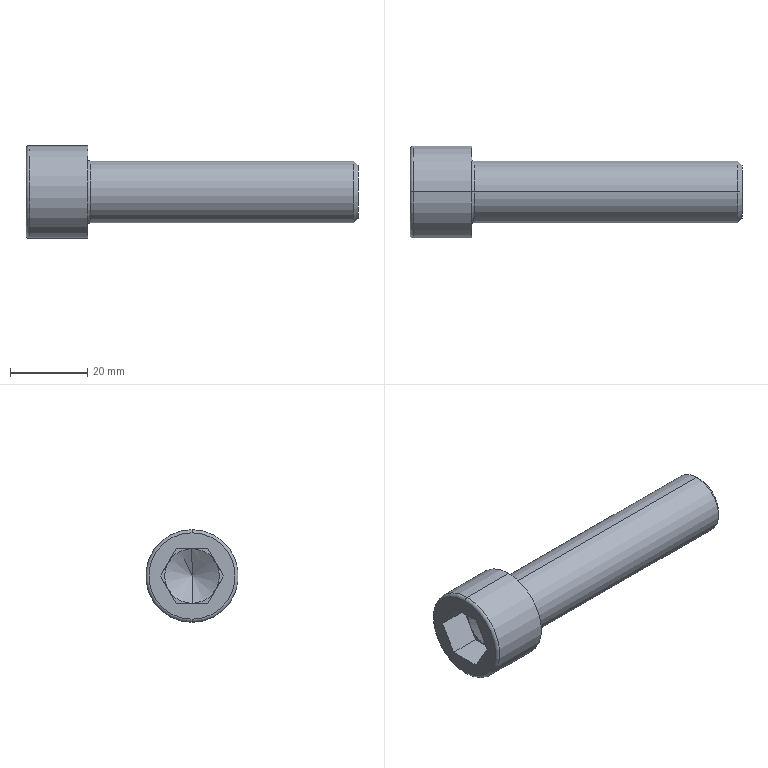Part | STEP file | PN_0053_socket head screw-M16x70L | 1 solid | 27 faces | box 86 x 24 x 24 mm | volume 19678 mm3 | plane 15 | cone 4 | torus 4 | cylinder 4 | commonest cylinder face diameters 16 x2 24 x2